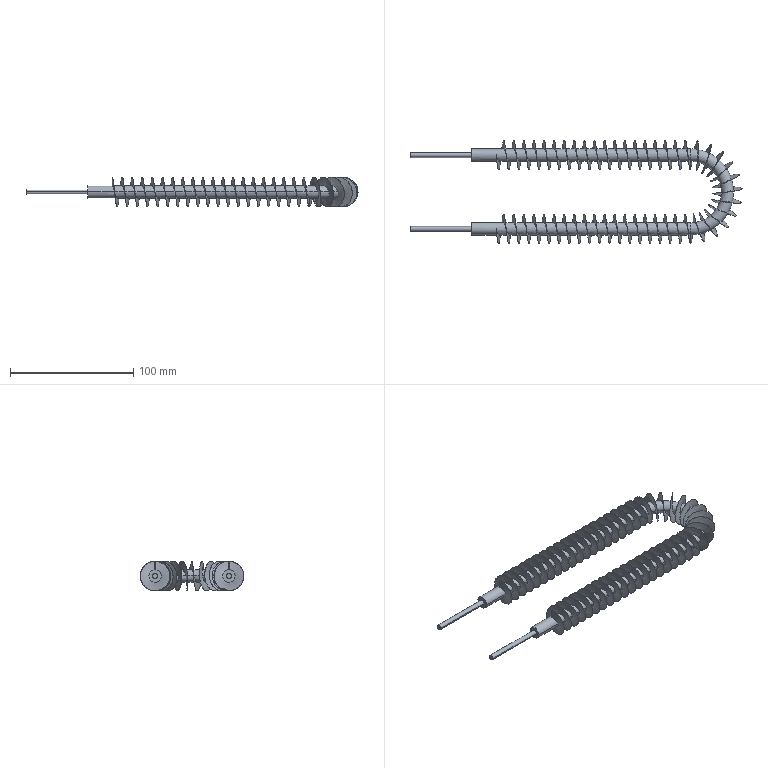Part | STEP file | 001 | 1 solid | 122 faces | box 269.918 x 84.021 x 24.021 mm | volume 38050 mm3 | cylinder 83 | torus 24 | spline 9 | plane 6 | commonest cylinder face diameters 10 x79 4 x4